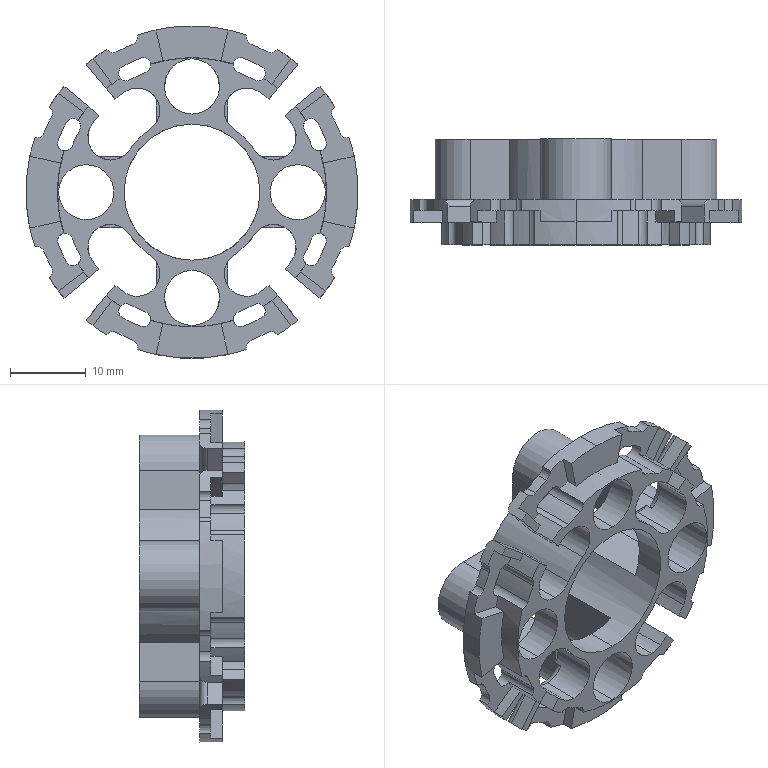Part | SolidWorks | features ICE 5, Extrusion 1, Fillet 1 | 1 solid | 245 faces | box 44 x 14 x 44 mm | volume 3465 mm3 | cylinder 141 | plane 86 | torus 18 | commonest cylinder face diameters 2 x52 35.6 x13 44 x13 6 x12 7.3 x8 32 x8